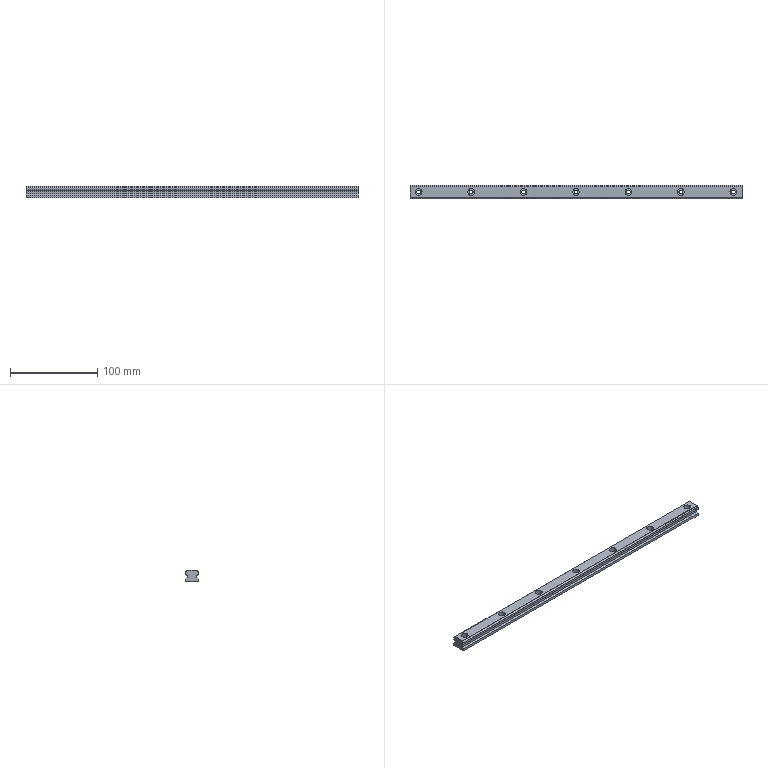Part | SolidWorks | features BaseBody 1 | 1 solid | 59 faces | box 380 x 15 x 13 mm | volume 63866 mm3 | cylinder 40 | plane 19 | commonest cylinder face diameters 4.5 x14 7.5 x14 0.28 x8 5.556 x4